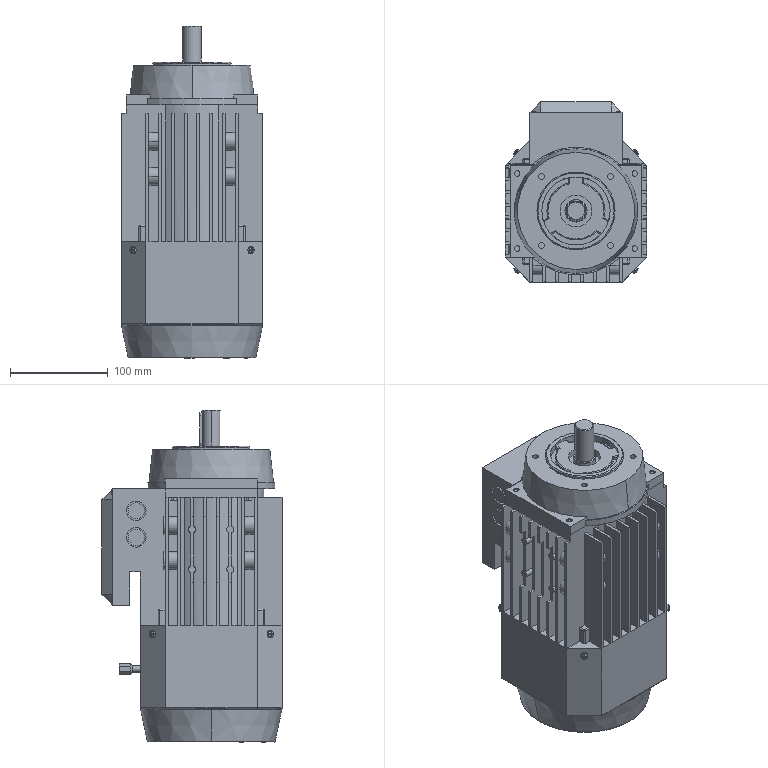Part | SolidWorks | features BaseBody 1 | 1 solid | 1226 faces | box 145.261 x 184.63 x 340 mm | volume 4951111 mm3 | plane 958 | cylinder 186 | spline 70 | cone 12 | commonest cylinder face diameters 108.75 x29 5.8 x24 7.25 x24 2 x20 18 x18 2.32 x12